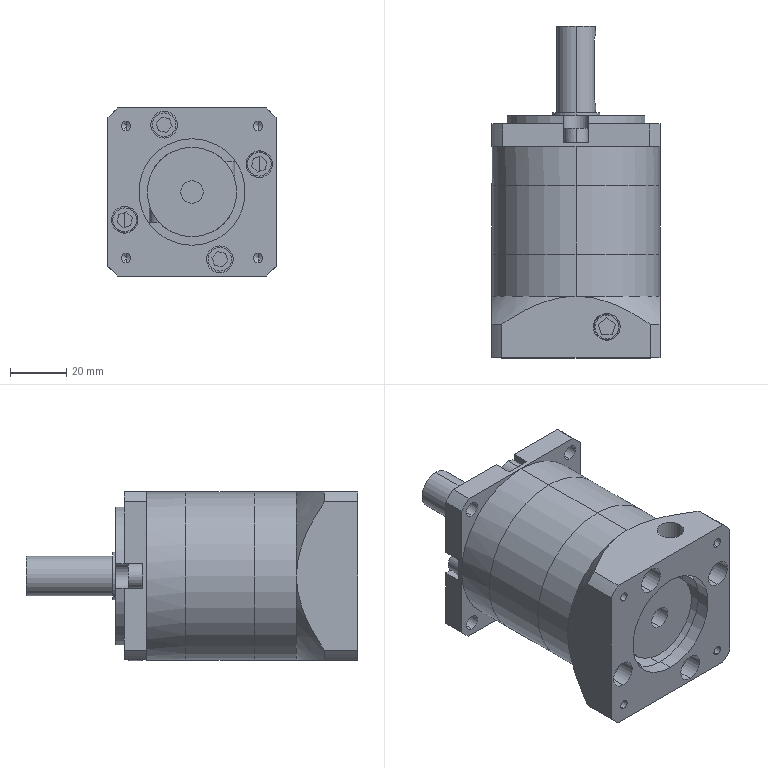Part | SolidWorks | features MBimport 1 | 4 solids | 260 faces | box 60.5 x 118.5 x 60.5 mm | volume 241824 mm3 | plane 149 | cylinder 97 | cone 14 | commonest cylinder face diameters 8.5 x20 3.3 x8 5.5 x8 9.5 x8 80 x8 9 x7